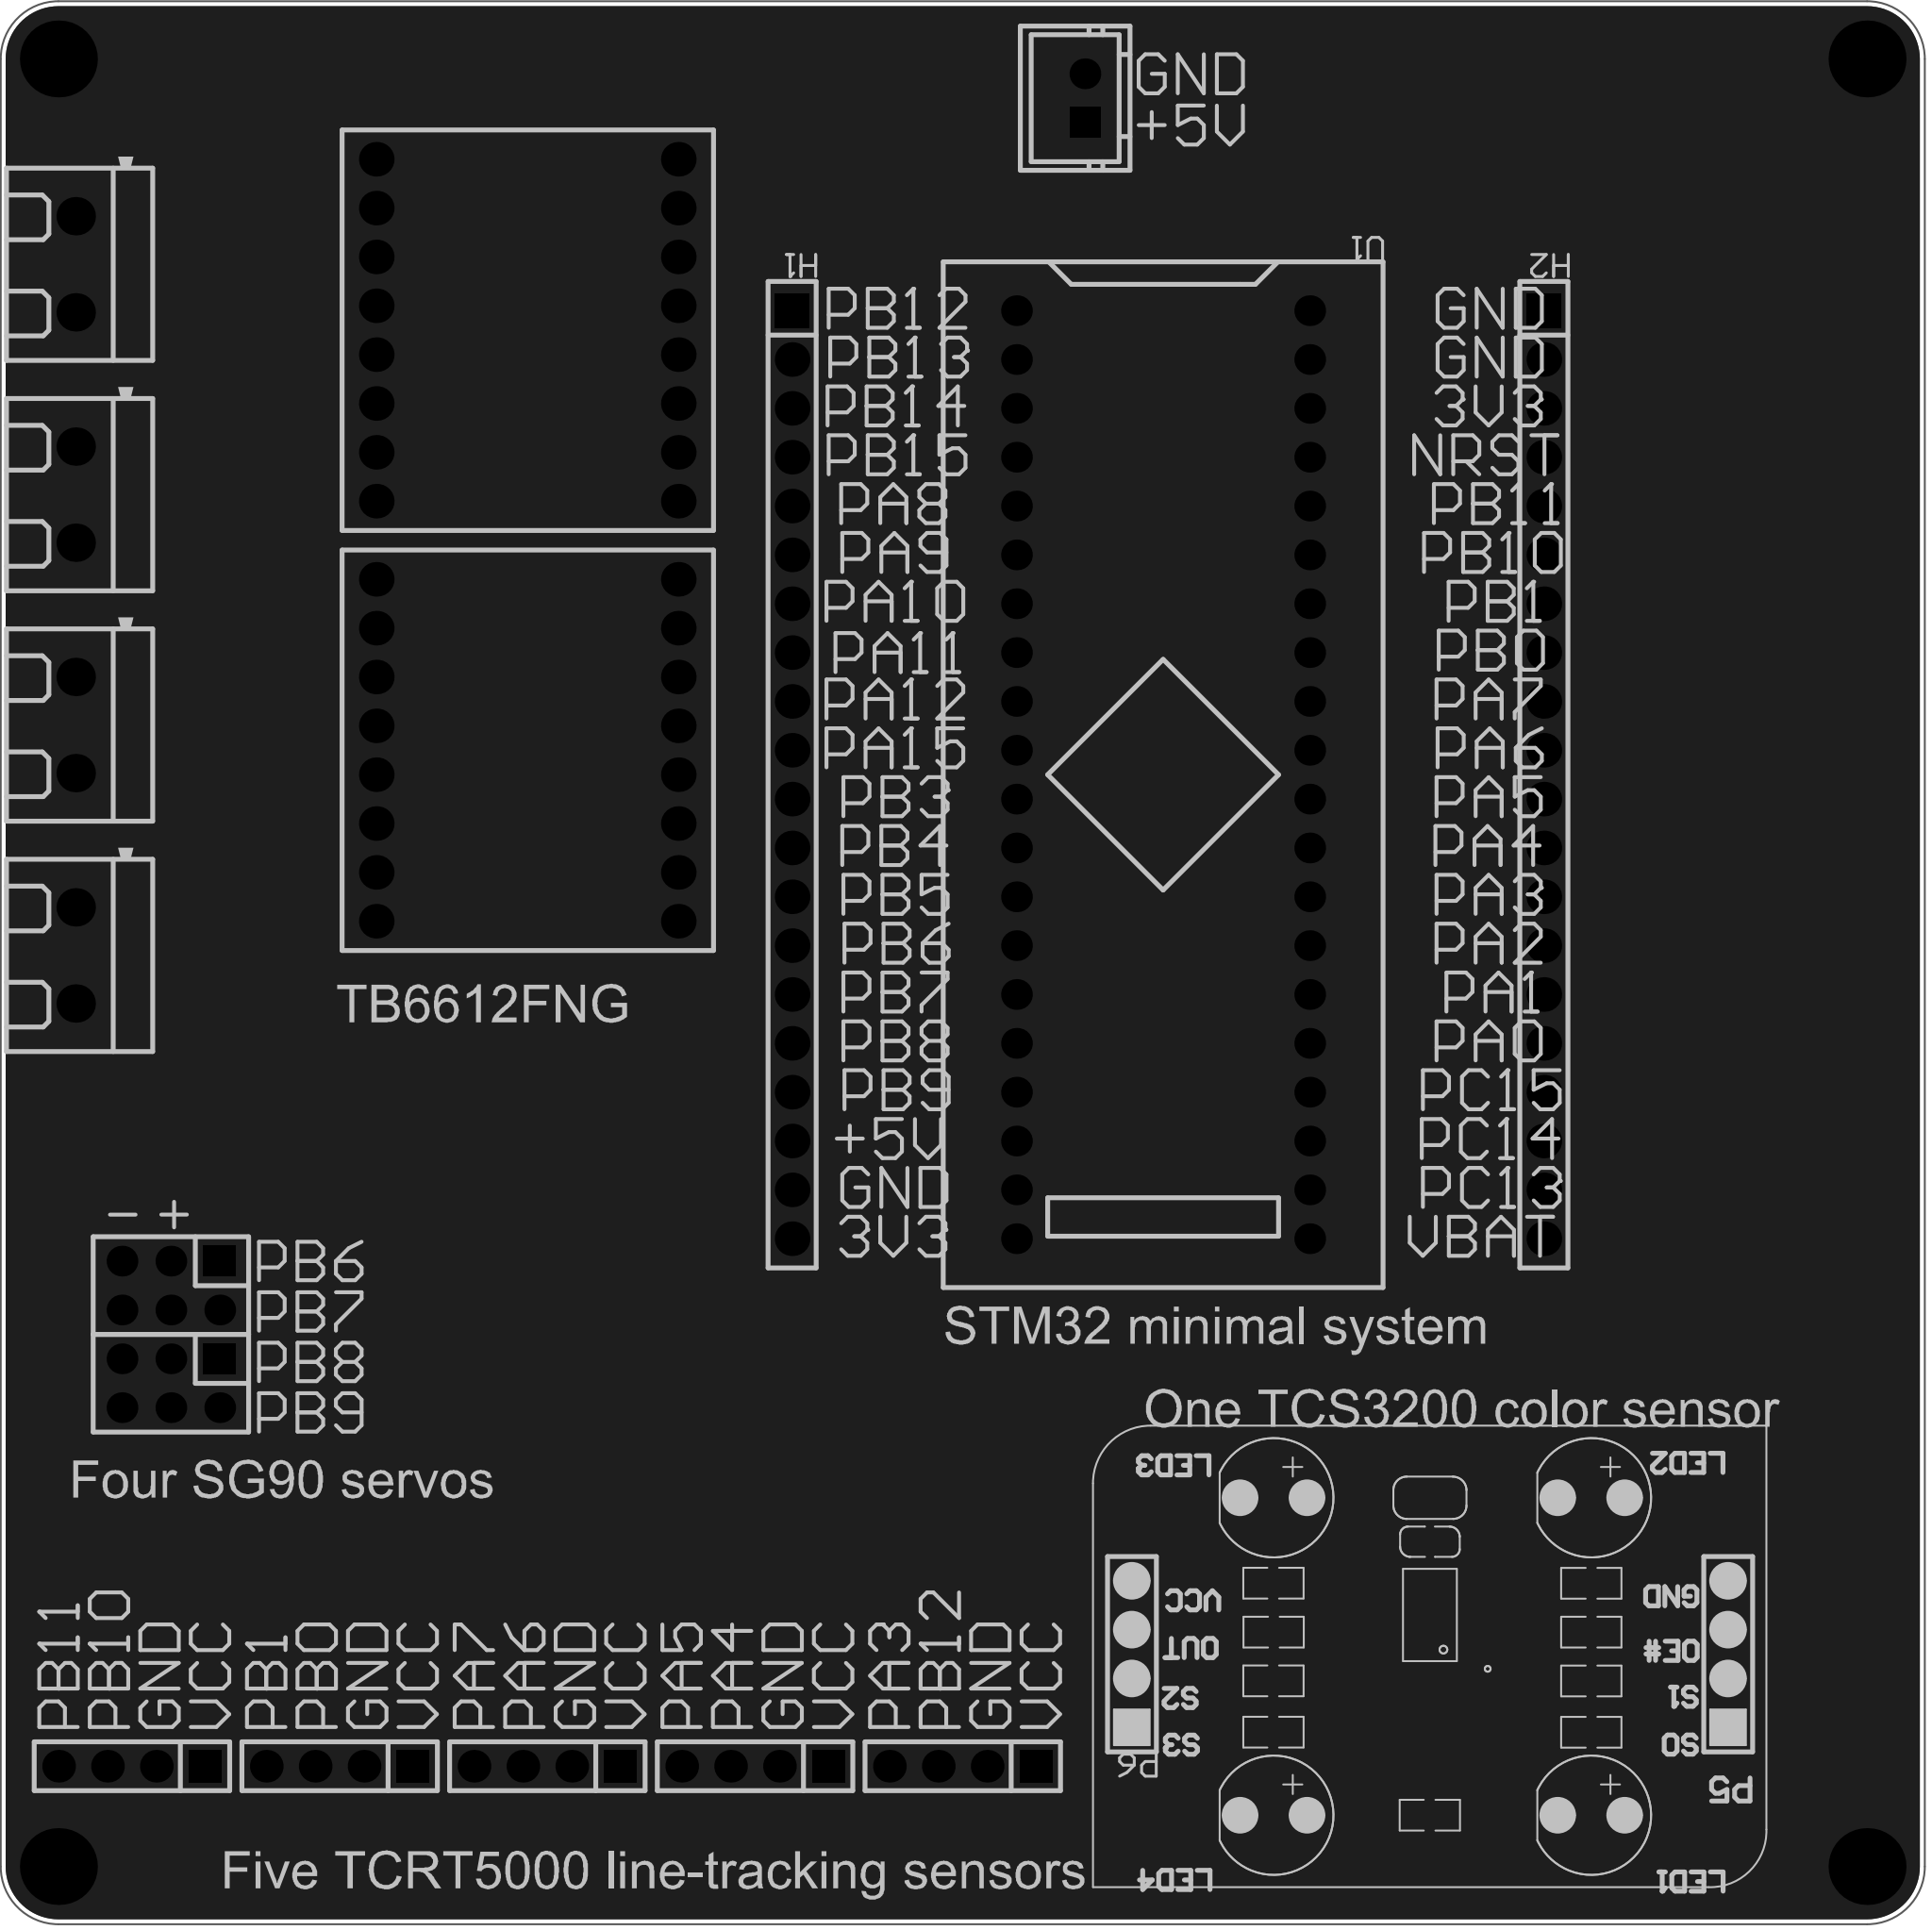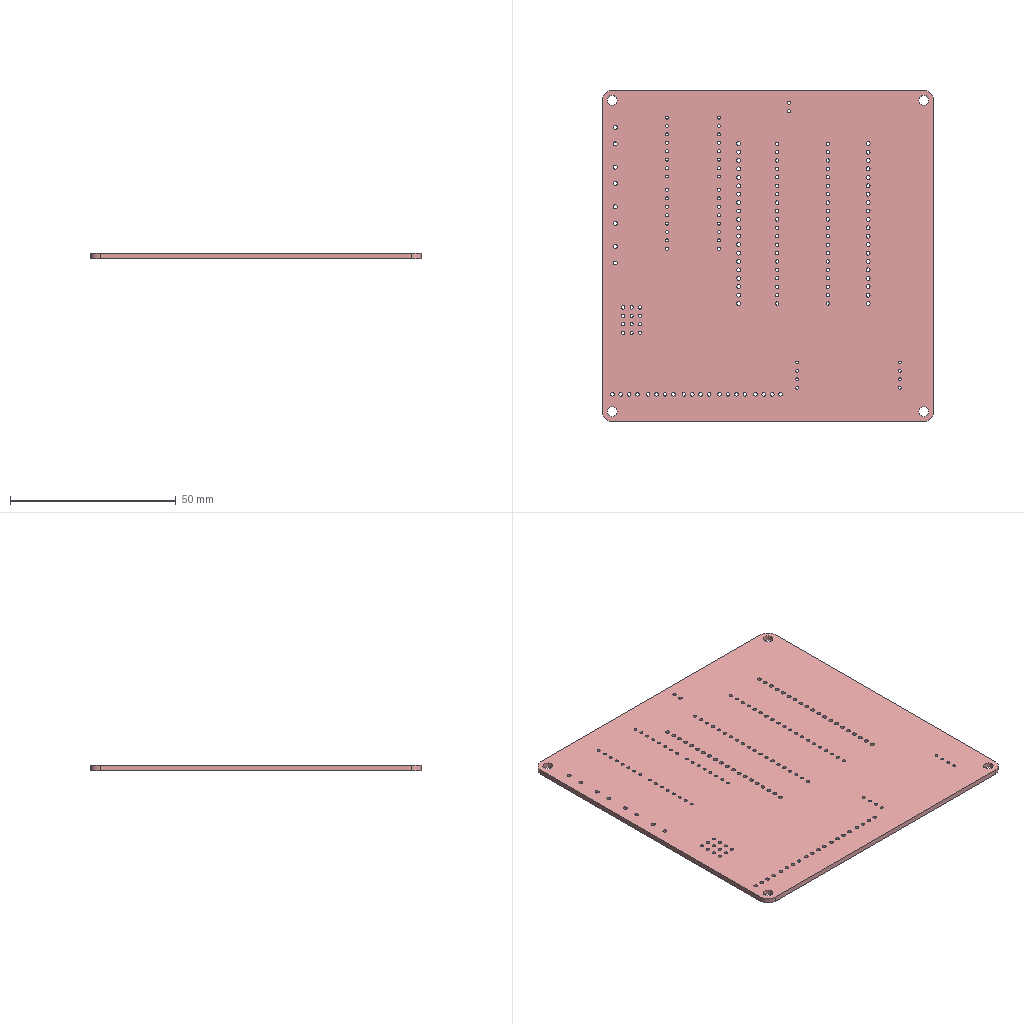Circuit board layout | Altium Designer | box 100 x 100 x 1.6 mm
Layer stack:
# Altium Designer layer stack of  (unit mm; dielectric type: 0 none, 1 core, 2 prepreg, 3 surface material)
index,name,kind,layer,copper_thickness_mm,dielectric_type,dielectric_thickness_mm,dielectric_material,dielectric_constant
0,Top Paste Mask Layer,other,,,,,,
1,Top Silkscreen Layer,other,,,,,,
2,Top Solder Mask Layer,dielectric,,,3,0.01,,3.3
3,Top Layer,copper,Top Layer,0.035,,,,
4,Dielectric1,dielectric,,,3,1.51,FR4,4.5
5,Bottom Layer,copper,Bottom Layer,0.035,,,,
6,Bottom Solder Mask Layer,dielectric,,,3,0.01,,3.3
7,Bottom Silkscreen Layer,other,,,,,,
8,Bottom Paste Mask Layer,other,,,,,,
# drill layer pairs: low layer,high layer
drill_pair,Top Layer,Bottom Layer
Part placement:
Designator,Comment,Layer,Footprint,Center-X(mm),Center-Y(mm),Rotation
U1,STM32F103C8T6-Card,TopLayer,CONN-TH_L53.3-W22.9_STM32F103C8T6-CARD,140.97,138.684,270
H1,,TopLayer,HDR-TH_20P-P2.54-V-F,121.687,138.684,270
H2,,TopLayer,HDR-TH_20P-P2.54-V-F,160.758,138.684,270
H22,,TopLayer,HDR-TH_6P-P2.54-V-F-R2-C3-S2.54,89.4,112.118,180
H23,,TopLayer,HDR-TH_6P-P2.54-V-F-R2-C3-S2.54,89.4,107.038,180
P1,KF301-2P terminal block,TopLayer,CONN-TH_XY301V-A-5.0-2P,84.455,141.266,90
P2,KF301-2P terminal block,TopLayer,CONN-TH_XY301V-A-5.0-2P,84.455,129.286,90
P3,KF301-2P terminal block,TopLayer,CONN-TH_XY301V-A-5.0-2P,84.455,165.227,90
P4,KF301-2P terminal block,TopLayer,CONN-TH_XY301V-A-5.0-2P,84.455,153.247,90
U3,,TopLayer,tb6612,107.925,139.954,0
U4,,TopLayer,tb6612,107.925,161.798,0
P5,2.54-1*4P_JX,TopLayer,2.54-1*4P_JX,170.338,92.946,90
P6,2.54-1*4P_JX,TopLayer,2.54-1*4P_JX,139.35,92.946,90
H24,,TopLayer,HDR-TH_4P-P2.54-V-M,87.376,87.122,180
H25,,TopLayer,HDR-TH_4P-P2.54-V-M,130.556,87.122,180
H26,,TopLayer,HDR-TH_4P-P2.54-V-M,119.761,87.122,180
H27,,TopLayer,HDR-TH_4P-P2.54-V-M,108.966,87.122,180
H28,,TopLayer,HDR-TH_4P-P2.54-V-M,98.171,87.122,180
U5,_x001F_XH2.54-2P,TopLayer,CONN-TH_2P-P2.54-V,136.906,173.863,90
Pad and via stacks:
# Altium Designer via and pad stacks of  (unit mm). Each distinct definition once, with the count of objects using it.
# via: kind,start_layer,end_layer,hole_mm,diameter_mm,mode(0 simple;1 top-mid-bottom;2 full stack),diameter_per_layer,count,example_net
# pad: kind,layer,hole_mm,hole_type(0 round;1 square;2 slot),plating,top_size,top_shape(1 round;2 rect;3 octagon;9 rounded rect),mid_size,bottom_size,mode,footprint,size_per_layer,count,example
pad,Multi-Layer,3,0,plated,4x4,1,4x4,4x4,0,,,4,1
pad,Multi-Layer,1,0,plated,1.6x1.6,1,1.6x1.6,1.6x1.6,0,CONN-TH_L53.3-W22.9_STM32F103C8T6-CARD,,40,U1.1
pad,Multi-Layer,1.2,0,plated,1.8x1.8,2,1.8x1.8,1.8x1.8,0,HDR-TH_20P-P2.54-V-F,,2,H1.1
pad,Multi-Layer,1.2,0,plated,1.8x1.8,1,1.8x1.8,1.8x1.8,0,HDR-TH_20P-P2.54-V-F,,38,H1.2
pad,Multi-Layer,1,0,plated,1.7x1.6,2,1.7x1.6,1.7x1.6,0,HDR-TH_6P-P2.54-V-F-R2-C3-S2.54,,2,H22.1
pad,Multi-Layer,1,0,plated,1.6x1.6,1,1.6x1.6,1.6x1.6,0,HDR-TH_6P-P2.54-V-F-R2-C3-S2.54,,10,H22.2
pad,Multi-Layer,1.2,0,plated,2x2,1,2x2,2x2,0,CONN-TH_XY301V-A-5.0-2P,,8,P1.1
pad,Multi-Layer,0.9,0,plated,1.8x1.8,1,1.8x1.8,1.8x1.8,0,tb6612,,32,U3.1
pad,Multi-Layer,0.889,0,plated,1.651x1.651,2,1.651x1.651,1.651x1.651,0,2.54-1*4P_JX,,2,P5.1
pad,Multi-Layer,0.889,0,plated,1.651x1.651,1,1.651x1.651,1.651x1.651,0,2.54-1*4P_JX,,6,P5.2
pad,Multi-Layer,1.1,0,plated,1.7x1.7,2,1.7x1.7,1.7x1.7,0,HDR-TH_4P-P2.54-V-M,,5,H24.1
pad,Multi-Layer,1.1,0,plated,1.7x1.7,1,1.7x1.7,1.7x1.7,0,HDR-TH_4P-P2.54-V-M,,15,H24.2
pad,Multi-Layer,1,0,plated,1.6x1.6,1,1.6x1.6,1.6x1.6,0,CONN-TH_2P-P2.54-V,,1,U5.2
pad,Multi-Layer,1,0,plated,1.6x1.6,2,1.6x1.6,1.6x1.6,0,CONN-TH_2P-P2.54-V,,1,U5.1
Copper pours:
name,layer,net,type(0 solid;1 hatched;2 none)
Bottom Layer-GND,Bottom Layer,GND,0
Top Layer-GND,Top Layer,GND,0